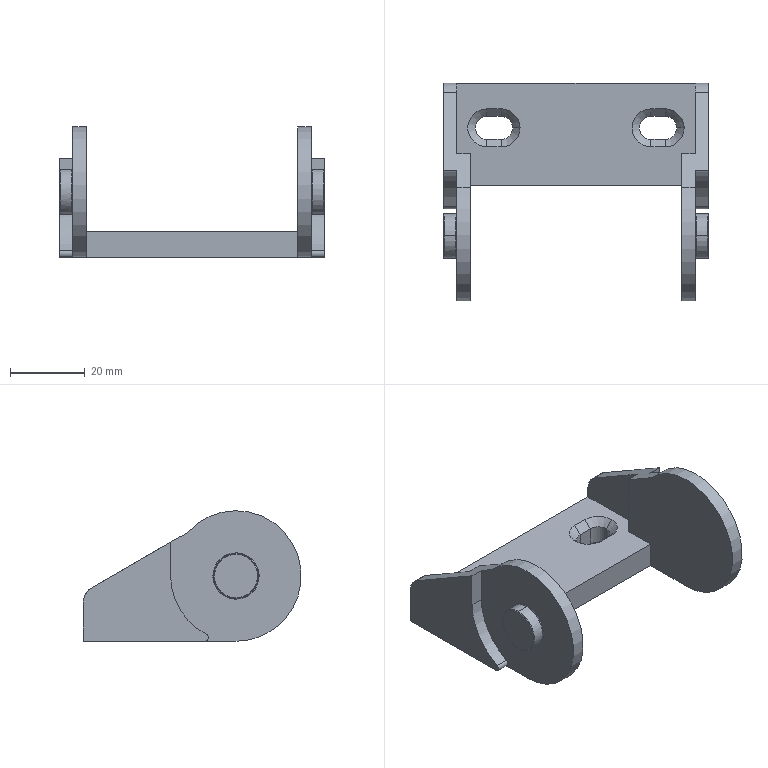Part | STEP file | TFH-FIX-END57 | 1 solid | 66 faces | box 71 x 58.5 x 35 mm | volume 23684 mm3 | plane 34 | cylinder 18 | torus 6 | cone 6 | spline 2 | commonest cylinder face diameters 6.2 x6 12 x4 35 x4 2 x2 10 x2